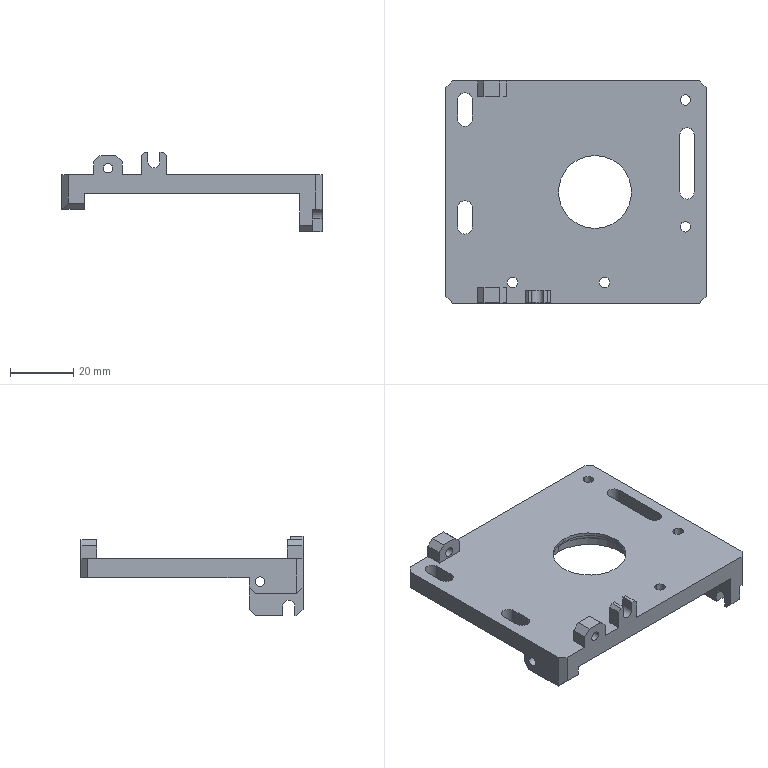NC program | NX | posted with a generic post | part box 82 x 70 x 25 mm
Lines 4706 to 5778 of 8354:
(FIXED_CONTOUR_COPY , TOOL : R1)
N9368 T02 M6
N9370 G54
N9372 G17 G0 G90 X-30.6 Y34.099 S9500 M3
N9374 G43 Z30. H2
N9376 Z2.8
N9378 G94 G1 Z0. F2800.
N9380 X-30.341 Z-0.034
N9382 X-30.1 Z-0.134
N9384 X-29.893 Z-0.293
N9386 X-29.734 Z-0.5
N9388 X-29.634 Z-0.741
N9390 X-29.6 Z-1.
N9392 Z-3.975
N9394 X-29.607 Z-4.096
N9396 X-29.613 Z-4.141
N9398 X-29.653 Z-4.278
N9400 X-29.706 Z-4.405
N9402 X-29.76 Z-4.502
N9404 X-29.813 Z-4.567
N9406 X-29.883 Z-4.646
N9408 X-29.953 Z-4.704
N9410 X-30.095 Z-4.794
N9412 X-30.233 Z-4.85
N9414 X-30.373 Z-4.889
N9416 X-30.517 Z-4.898
N9418 X-30.653 Z-4.885
N9420 X-30.793 Z-4.842
N9422 X-30.933 Z-4.779
N9424 X-31.003 Z-4.74
N9426 X-31.073 Z-4.682
N9428 X-31.143 Z-4.621
N9430 X-31.213 Z-4.536
N9432 X-31.306 Z-4.381
N9434 X-31.353 Z-4.256
N9436 X-31.377 Z-4.179
N9438 X-31.388 Z-4.13
N9440 X-31.394 Z-4.09
N9442 X-31.4 Z-3.975
N9444 Z-1.61
N9446 Y34.123 Z-1.
N9448 Y34.199
N9450 Z-3.975
N9452 X-31.394 Z-4.09
N9454 X-31.388 Z-4.13
N9456 X-31.377 Z-4.179
N9458 X-31.353 Z-4.256
N9460 X-31.306 Z-4.381
N9462 X-31.213 Z-4.536
N9464 X-31.143 Z-4.621
N9466 X-31.073 Z-4.682
N9468 X-31.003 Z-4.74
N9470 X-30.933 Z-4.779
N9472 X-30.793 Z-4.842
N9474 X-30.653 Z-4.885
N9476 X-30.513 Z-4.898
N9478 X-30.373 Z-4.889
N9480 X-30.233 Z-4.85
N9482 X-30.094 Z-4.793
N9484 X-29.953 Z-4.704
N9486 X-29.883 Z-4.646
N9488 X-29.813 Z-4.567
N9490 X-29.76 Z-4.502
N9492 X-29.706 Z-4.405
N9494 X-29.653 Z-4.278
N9496 X-29.613 Z-4.141
N9498 X-29.607 Z-4.096
N9500 X-29.6 Z-3.975
N9502 Z-1.
N9504 Y34.299
N9506 Z-3.975
N9508 X-29.607 Z-4.096
N9510 X-29.613 Z-4.141
N9512 X-29.653 Z-4.278
N9514 X-29.706 Z-4.405
N9516 X-29.76 Z-4.502
N9518 X-29.813 Z-4.567
N9520 X-29.883 Z-4.646
N9522 X-29.953 Z-4.704
N9524 X-30.093 Z-4.793
N9526 X-30.233 Z-4.85
N9528 X-30.373 Z-4.889
N9530 X-30.513 Z-4.898
N9532 X-30.653 Z-4.885
N9534 X-30.793 Z-4.842
N9536 X-30.933 Z-4.779
N9538 X-31.003 Z-4.74
N9540 X-31.073 Z-4.682
N9542 X-31.143 Z-4.621
N9544 X-31.213 Z-4.536
N9546 X-31.306 Z-4.381
N9548 X-31.353 Z-4.256
N9550 X-31.377 Z-4.179
N9552 X-31.388 Z-4.13
N9554 X-31.394 Z-4.09
N9556 X-31.4 Z-3.975
N9558 Z-1.
N9560 Y34.399
N9562 Z-3.975
N9564 X-31.394 Z-4.09
N9566 X-31.388 Z-4.13
N9568 X-31.377 Z-4.179
N9570 X-31.353 Z-4.256
N9572 X-31.306 Z-4.381
N9574 X-31.213 Z-4.536
N9576 X-31.143 Z-4.621
N9578 X-31.073 Z-4.682
N9580 X-31.003 Z-4.74
N9582 X-30.933 Z-4.779
N9584 X-30.793 Z-4.842
N9586 X-30.653 Z-4.885
N9588 X-30.513 Z-4.898
N9590 X-30.373 Z-4.889
N9592 X-30.233 Z-4.85
N9594 X-30.093 Z-4.793
N9596 X-29.953 Z-4.704
N9598 X-29.883 Z-4.646
N9600 X-29.813 Z-4.567
N9602 X-29.76 Z-4.502
N9604 X-29.706 Z-4.405
N9606 X-29.653 Z-4.278
N9608 X-29.613 Z-4.141
N9610 X-29.607 Z-4.096
N9612 X-29.6 Z-3.975
N9614 Z-1.
N9616 Y34.499
N9618 Z-3.975
N9620 X-29.607 Z-4.096
N9622 X-29.613 Z-4.141
N9624 X-29.653 Z-4.278
N9626 X-29.706 Z-4.405
N9628 X-29.76 Z-4.502
N9630 X-29.813 Z-4.567
N9632 X-29.883 Z-4.646
N9634 X-29.953 Z-4.704
N9636 X-30.093 Z-4.793
N9638 X-30.233 Z-4.85
N9640 X-30.373 Z-4.889
N9642 X-30.513 Z-4.898
N9644 X-30.653 Z-4.885
N9646 X-30.793 Z-4.842
N9648 X-30.933 Z-4.779
N9650 X-31.003 Z-4.74
N9652 X-31.073 Z-4.682
N9654 X-31.143 Z-4.621
N9656 X-31.213 Z-4.536
N9658 X-31.306 Z-4.381
N9660 X-31.353 Z-4.256
N9662 X-31.377 Z-4.179
N9664 X-31.388 Z-4.13
N9666 X-31.394 Z-4.09
N9668 X-31.4 Z-3.975
N9670 Z-1.
N9672 Y34.599
N9674 Z-3.975
N9676 X-31.394 Z-4.09
N9678 X-31.388 Z-4.13
N9680 X-31.377 Z-4.179
N9682 X-31.353 Z-4.256
N9684 X-31.306 Z-4.381
N9686 X-31.213 Z-4.536
N9688 X-31.143 Z-4.621
N9690 X-31.073 Z-4.682
N9692 X-31.003 Z-4.74
N9694 X-30.933 Z-4.779
N9696 X-30.793 Z-4.842
N9698 X-30.653 Z-4.885
N9700 X-30.513 Z-4.898
N9702 X-30.373 Z-4.889
N9704 X-30.233 Z-4.85
N9706 X-30.093 Z-4.793
N9708 X-29.953 Z-4.704
N9710 X-29.883 Z-4.646
N9712 X-29.813 Z-4.567
N9714 X-29.76 Z-4.502
N9716 X-29.706 Z-4.405
N9718 X-29.653 Z-4.278
N9720 X-29.613 Z-4.141
N9722 X-29.607 Z-4.096
N9724 X-29.6 Z-3.975
N9726 Z-1.
N9728 Y34.699
N9730 Z-3.975
N9732 X-29.607 Z-4.096
N9734 X-29.613 Z-4.141
N9736 X-29.653 Z-4.278
N9738 X-29.706 Z-4.405
N9740 X-29.76 Z-4.502
N9742 X-29.813 Z-4.567
N9744 X-29.883 Z-4.646
N9746 X-29.953 Z-4.704
N9748 X-30.093 Z-4.793
N9750 X-30.233 Z-4.85
N9752 X-30.373 Z-4.889
N9754 X-30.513 Z-4.898
N9756 X-30.653 Z-4.885
N9758 X-30.793 Z-4.842
N9760 X-30.933 Z-4.779
N9762 X-31.003 Z-4.74
N9764 X-31.073 Z-4.682
N9766 X-31.143 Z-4.621
N9768 X-31.213 Z-4.536
N9770 X-31.306 Z-4.381
N9772 X-31.353 Z-4.256
N9774 X-31.377 Z-4.179
N9776 X-31.388 Z-4.13
N9778 X-31.394 Z-4.09
N9780 X-31.4 Z-3.975
N9782 Z-1.
N9784 Y34.799
N9786 Z-3.975
N9788 X-31.394 Z-4.09
N9790 X-31.388 Z-4.13
N9792 X-31.377 Z-4.179
N9794 X-31.353 Z-4.256
N9796 X-31.306 Z-4.381
N9798 X-31.213 Z-4.536
N9800 X-31.143 Z-4.621
N9802 X-31.073 Z-4.682
N9804 X-31.003 Z-4.74
N9806 X-30.933 Z-4.779
N9808 X-30.793 Z-4.842
N9810 X-30.653 Z-4.885
N9812 X-30.513 Z-4.898
N9814 X-30.373 Z-4.889
N9816 X-30.233 Z-4.85
N9818 X-30.093 Z-4.793
N9820 X-29.953 Z-4.704
N9822 X-29.883 Z-4.646
N9824 X-29.813 Z-4.567
N9826 X-29.76 Z-4.502
N9828 X-29.706 Z-4.405
N9830 X-29.653 Z-4.278
N9832 X-29.613 Z-4.141
N9834 X-29.607 Z-4.096
N9836 X-29.6 Z-3.975
N9838 Z-1.
N9840 Y34.899
N9842 Z-3.975
N9844 X-29.607 Z-4.096
N9846 X-29.613 Z-4.141
N9848 X-29.653 Z-4.278
N9850 X-29.706 Z-4.405
N9852 X-29.76 Z-4.502
N9854 X-29.813 Z-4.567
N9856 X-29.883 Z-4.646
N9858 X-29.953 Z-4.704
N9860 X-30.093 Z-4.793
N9862 X-30.233 Z-4.85
N9864 X-30.373 Z-4.889
N9866 X-30.513 Z-4.898
N9868 X-30.653 Z-4.885
N9870 X-30.793 Z-4.842
N9872 X-30.933 Z-4.779
N9874 X-31.003 Z-4.74
N9876 X-31.073 Z-4.682
N9878 X-31.143 Z-4.621
N9880 X-31.213 Z-4.536
N9882 X-31.306 Z-4.381
N9884 X-31.353 Z-4.256
N9886 X-31.377 Z-4.179
N9888 X-31.388 Z-4.13
N9890 X-31.394 Z-4.09
N9892 X-31.4 Z-3.975
N9894 Z-1.
N9896 Y34.999
N9898 Z-3.975
N9900 X-31.394 Z-4.09
N9902 X-31.388 Z-4.13
N9904 X-31.377 Z-4.179
N9906 X-31.353 Z-4.256
N9908 X-31.306 Z-4.381
N9910 X-31.213 Z-4.536
N9912 X-31.143 Z-4.621
N9914 X-31.073 Z-4.682
N9916 X-31.003 Z-4.74
N9918 X-30.933 Z-4.779
N9920 X-30.793 Z-4.842
N9922 X-30.653 Z-4.885
N9924 X-30.513 Z-4.898
N9926 X-30.373 Z-4.889
N9928 X-30.233 Z-4.85
N9930 X-30.093 Z-4.793
N9932 X-29.953 Z-4.704
N9934 X-29.883 Z-4.646
N9936 X-29.813 Z-4.567
N9938 X-29.76 Z-4.502
N9940 X-29.706 Z-4.405
N9942 X-29.653 Z-4.278
N9944 X-29.613 Z-4.141
N9946 X-29.607 Z-4.096
N9948 X-29.6 Z-3.975
N9950 Z-1.
N9952 Y35.099
N9954 Z-3.975
N9956 X-29.607 Z-4.096
N9958 X-29.613 Z-4.141
N9960 X-29.653 Z-4.278
N9962 X-29.706 Z-4.405
N9964 X-29.76 Z-4.502
N9966 X-29.813 Z-4.567
N9968 X-29.883 Z-4.646
N9970 X-29.953 Z-4.704
N9972 X-30.093 Z-4.793
N9974 X-30.233 Z-4.85
N9976 X-30.373 Z-4.889
N9978 X-30.513 Z-4.898
N9980 X-30.653 Z-4.885
N9982 X-30.793 Z-4.842
N9984 X-30.933 Z-4.779
N9986 X-31.003 Z-4.74
N9988 X-31.073 Z-4.682
N9990 X-31.143 Z-4.621
N9992 X-31.213 Z-4.536
N9994 X-31.306 Z-4.381
N9996 X-31.353 Z-4.256
N9998 X-31.377 Z-4.179
N10000 X-31.388 Z-4.13
N10002 X-31.394 Z-4.09
N10004 X-31.4 Z-3.975
N10006 Z-1.
N10008 Y35.199
N10010 Z-3.975
N10012 X-31.394 Z-4.09
N10014 X-31.388 Z-4.13
N10016 X-31.377 Z-4.179
N10018 X-31.353 Z-4.256
N10020 X-31.306 Z-4.381
N10022 X-31.213 Z-4.536
N10024 X-31.143 Z-4.621
N10026 X-31.073 Z-4.682
N10028 X-31.003 Z-4.74
N10030 X-30.933 Z-4.779
N10032 X-30.793 Z-4.842
N10034 X-30.653 Z-4.885
N10036 X-30.513 Z-4.898
N10038 X-30.373 Z-4.889
N10040 X-30.233 Z-4.85
N10042 X-30.093 Z-4.793
N10044 X-29.953 Z-4.704
N10046 X-29.883 Z-4.646
N10048 X-29.813 Z-4.567
N10050 X-29.76 Z-4.502
N10052 X-29.706 Z-4.405
N10054 X-29.653 Z-4.278
N10056 X-29.613 Z-4.141
N10058 X-29.607 Z-4.096
N10060 X-29.6 Z-3.975
N10062 Z-1.
N10064 Y35.299
N10066 Z-3.975
N10068 X-29.607 Z-4.096
N10070 X-29.613 Z-4.141
N10072 X-29.653 Z-4.278
N10074 X-29.706 Z-4.405
N10076 X-29.76 Z-4.502
N10078 X-29.813 Z-4.567
N10080 X-29.883 Z-4.646
N10082 X-29.953 Z-4.704
N10084 X-30.093 Z-4.793
N10086 X-30.233 Z-4.85
N10088 X-30.373 Z-4.889
N10090 X-30.513 Z-4.898
N10092 X-30.653 Z-4.885
N10094 X-30.793 Z-4.842
N10096 X-30.933 Z-4.779
N10098 X-31.003 Z-4.74
N10100 X-31.073 Z-4.682
N10102 X-31.143 Z-4.621
N10104 X-31.213 Z-4.536
N10106 X-31.306 Z-4.381
N10108 X-31.353 Z-4.256
N10110 X-31.377 Z-4.179
N10112 X-31.388 Z-4.13
N10114 X-31.394 Z-4.09
N10116 X-31.4 Z-3.975
N10118 Z-1.
N10120 Y35.399
N10122 Z-3.975
N10124 X-31.394 Z-4.09
N10126 X-31.388 Z-4.129
N10128 X-31.377 Z-4.178
N10130 X-31.353 Z-4.256
N10132 X-31.306 Z-4.381
N10134 X-31.213 Z-4.536
N10136 X-31.143 Z-4.621
N10138 X-31.075 Z-4.681
N10140 X-31.003 Z-4.74
N10142 X-30.933 Z-4.779
N10144 X-30.793 Z-4.842
N10146 X-30.653 Z-4.885
N10148 X-30.513 Z-4.898
N10150 X-30.373 Z-4.889
N10152 X-30.233 Z-4.85
N10154 X-30.093 Z-4.793
N10156 X-29.953 Z-4.704
N10158 X-29.883 Z-4.646
N10160 X-29.815 Z-4.569
N10162 X-29.76 Z-4.502
N10164 X-29.706 Z-4.405
N10166 X-29.653 Z-4.278
N10168 X-29.613 Z-4.141
N10170 X-29.607 Z-4.097
N10172 X-29.6 Z-3.976
N10174 Z-1.
N10176 Y35.499
N10178 Z-3.975
N10180 X-29.607 Z-4.096
N10182 X-29.613 Z-4.141
N10184 X-29.653 Z-4.278
N10186 X-29.706 Z-4.405
N10188 X-29.76 Z-4.502
N10190 X-29.813 Z-4.567
N10192 X-29.883 Z-4.646
N10194 X-29.953 Z-4.704
N10196 X-30.093 Z-4.793
N10198 X-30.233 Z-4.85
N10200 X-30.373 Z-4.889
N10202 X-30.513 Z-4.898
N10204 X-30.653 Z-4.885
N10206 X-30.793 Z-4.842
N10208 X-30.933 Z-4.779
N10210 X-31.003 Z-4.74
N10212 X-31.073 Z-4.682
N10214 X-31.143 Z-4.621
N10216 X-31.213 Z-4.536
N10218 X-31.306 Z-4.381
N10220 X-31.353 Z-4.256
N10222 X-31.377 Z-4.179
N10224 X-31.388 Z-4.13
N10226 X-31.394 Z-4.09
N10228 X-31.4 Z-3.975
N10230 Z-1.
N10232 Y35.599
N10234 Z-3.975
N10236 X-31.394 Z-4.09
N10238 X-31.388 Z-4.13
N10240 X-31.377 Z-4.179
N10242 X-31.353 Z-4.256
N10244 X-31.306 Z-4.381
N10246 X-31.213 Z-4.536
N10248 X-31.143 Z-4.621
N10250 X-31.073 Z-4.682
N10252 X-31.003 Z-4.74
N10254 X-30.933 Z-4.779
N10256 X-30.793 Z-4.842
N10258 X-30.653 Z-4.885
N10260 X-30.513 Z-4.898
N10262 X-30.373 Z-4.889
N10264 X-30.233 Z-4.85
N10266 X-30.093 Z-4.793
N10268 X-29.953 Z-4.704
N10270 X-29.883 Z-4.646
N10272 X-29.813 Z-4.567
N10274 X-29.76 Z-4.502
N10276 X-29.706 Z-4.405
N10278 X-29.653 Z-4.278
N10280 X-29.613 Z-4.141
N10282 X-29.607 Z-4.096
N10284 X-29.6 Z-3.975
N10286 Z-1.
N10288 Y35.699
N10290 Z-3.975
N10292 X-29.607 Z-4.096
N10294 X-29.613 Z-4.141
N10296 X-29.653 Z-4.278
N10298 X-29.706 Z-4.405
N10300 X-29.76 Z-4.502
N10302 X-29.813 Z-4.567
N10304 X-29.883 Z-4.646
N10306 X-29.953 Z-4.704
N10308 X-30.093 Z-4.793
N10310 X-30.233 Z-4.85
N10312 X-30.373 Z-4.889
N10314 X-30.513 Z-4.898
N10316 X-30.653 Z-4.885
N10318 X-30.793 Z-4.842
N10320 X-30.933 Z-4.779
N10322 X-31.003 Z-4.74
N10324 X-31.073 Z-4.682
N10326 X-31.143 Z-4.621
N10328 X-31.213 Z-4.536
N10330 X-31.306 Z-4.381
N10332 X-31.353 Z-4.256
N10334 X-31.377 Z-4.179
N10336 X-31.388 Z-4.13
N10338 X-31.394 Z-4.09
N10340 X-31.4 Z-3.975
N10342 Z-1.
N10344 Y35.799
N10346 Z-3.975
N10348 X-31.394 Z-4.09
N10350 X-31.388 Z-4.13
N10352 X-31.377 Z-4.179
N10354 X-31.353 Z-4.256
N10356 X-31.306 Z-4.381
N10358 X-31.213 Z-4.536
N10360 X-31.143 Z-4.621
N10362 X-31.073 Z-4.682
N10364 X-31.003 Z-4.74
N10366 X-30.933 Z-4.779
N10368 X-30.793 Z-4.842
N10370 X-30.653 Z-4.885
N10372 X-30.513 Z-4.898
N10374 X-30.373 Z-4.889
N10376 X-30.233 Z-4.85
N10378 X-30.093 Z-4.793
N10380 X-29.953 Z-4.704
N10382 X-29.883 Z-4.646
N10384 X-29.813 Z-4.567
N10386 X-29.76 Z-4.502
N10388 X-29.706 Z-4.405
N10390 X-29.653 Z-4.278
N10392 X-29.613 Z-4.141
N10394 X-29.607 Z-4.096
N10396 X-29.6 Z-3.975
N10398 Z-1.
N10400 Y35.899
N10402 Z-3.975
N10404 X-29.607 Z-4.096
N10406 X-29.613 Z-4.141
N10408 X-29.653 Z-4.278
N10410 X-29.706 Z-4.405
N10412 X-29.76 Z-4.502
N10414 X-29.813 Z-4.567
N10416 X-29.883 Z-4.646
N10418 X-29.953 Z-4.704
N10420 X-30.093 Z-4.793
N10422 X-30.233 Z-4.85
N10424 X-30.373 Z-4.889
N10426 X-30.513 Z-4.898
N10428 X-30.653 Z-4.885
N10430 X-30.793 Z-4.842
N10432 X-30.933 Z-4.779
N10434 X-31.003 Z-4.74
N10436 X-31.073 Z-4.682
N10438 X-31.143 Z-4.621
N10440 X-31.213 Z-4.536
N10442 X-31.306 Z-4.381
N10444 X-31.353 Z-4.256
N10446 X-31.377 Z-4.179
N10448 X-31.388 Z-4.13
N10450 X-31.394 Z-4.09
N10452 X-31.4 Z-3.975
N10454 Z-1.
N10456 Y35.999
N10458 Z-3.975
N10460 X-31.394 Z-4.09
N10462 X-31.388 Z-4.13
N10464 X-31.377 Z-4.179
N10466 X-31.353 Z-4.256
N10468 X-31.306 Z-4.381
N10470 X-31.213 Z-4.536
N10472 X-31.143 Z-4.621
N10474 X-31.073 Z-4.682
N10476 X-31.003 Z-4.74
N10478 X-30.933 Z-4.779
N10480 X-30.793 Z-4.842
N10482 X-30.653 Z-4.885
N10484 X-30.513 Z-4.898
N10486 X-30.373 Z-4.889
N10488 X-30.233 Z-4.85
N10490 X-30.093 Z-4.793
N10492 X-29.953 Z-4.704
N10494 X-29.883 Z-4.646
N10496 X-29.813 Z-4.567
N10498 X-29.76 Z-4.502
N10500 X-29.706 Z-4.405
N10502 X-29.653 Z-4.278
N10504 X-29.613 Z-4.141
N10506 X-29.607 Z-4.096
N10508 X-29.6 Z-3.975
N10510 Z-1.
N10512 Y36.099
N10514 Z-3.975
N10516 X-29.607 Z-4.096
N10518 X-29.613 Z-4.141
N10520 X-29.653 Z-4.278
N10522 X-29.706 Z-4.405
N10524 X-29.76 Z-4.502
N10526 X-29.813 Z-4.567
N10528 X-29.883 Z-4.646
N10530 X-29.953 Z-4.704
N10532 X-30.093 Z-4.793
N10534 X-30.233 Z-4.85
N10536 X-30.373 Z-4.889
N10538 X-30.513 Z-4.898
N10540 X-30.653 Z-4.885
N10542 X-30.793 Z-4.842
N10544 X-30.933 Z-4.779
N10546 X-31.003 Z-4.74
N10548 X-31.073 Z-4.682
N10550 X-31.143 Z-4.621
N10552 X-31.213 Z-4.536
N10554 X-31.306 Z-4.381
N10556 X-31.353 Z-4.256
N10558 X-31.377 Z-4.179
N10560 X-31.388 Z-4.13
N10562 X-31.394 Z-4.09
N10564 X-31.4 Z-3.975
N10566 Z-1.
N10568 Y36.199
N10570 Z-3.975
N10572 X-31.394 Z-4.09
N10574 X-31.388 Z-4.13
N10576 X-31.377 Z-4.179
N10578 X-31.353 Z-4.256
N10580 X-31.306 Z-4.381
N10582 X-31.213 Z-4.536
N10584 X-31.143 Z-4.621
N10586 X-31.073 Z-4.682
N10588 X-31.003 Z-4.74
N10590 X-30.933 Z-4.779
N10592 X-30.793 Z-4.842
N10594 X-30.653 Z-4.885
N10596 X-30.513 Z-4.898
N10598 X-30.373 Z-4.889
N10600 X-30.233 Z-4.85
N10602 X-30.093 Z-4.793
N10604 X-29.953 Z-4.704
N10606 X-29.883 Z-4.646
N10608 X-29.813 Z-4.567
N10610 X-29.76 Z-4.502
N10612 X-29.706 Z-4.405
N10614 X-29.653 Z-4.278
N10616 X-29.613 Z-4.141
N10618 X-29.607 Z-4.096
N10620 X-29.6 Z-3.975
N10622 Z-1.
N10624 Y36.299
N10626 Z-3.975
N10628 X-29.607 Z-4.096
N10630 X-29.613 Z-4.141
N10632 X-29.653 Z-4.278
N10634 X-29.706 Z-4.405
N10636 X-29.76 Z-4.502
N10638 X-29.813 Z-4.567
N10640 X-29.883 Z-4.646
N10642 X-29.953 Z-4.704
N10644 X-30.093 Z-4.793
N10646 X-30.233 Z-4.85
N10648 X-30.373 Z-4.889
N10650 X-30.513 Z-4.898
N10652 X-30.653 Z-4.885
N10654 X-30.793 Z-4.842
N10656 X-30.933 Z-4.779
N10658 X-31.003 Z-4.74
N10660 X-31.073 Z-4.682
N10662 X-31.143 Z-4.621
N10664 X-31.213 Z-4.536
N10666 X-31.306 Z-4.381
N10668 X-31.353 Z-4.256
N10670 X-31.377 Z-4.179
N10672 X-31.388 Z-4.13
N10674 X-31.394 Z-4.09
N10676 X-31.4 Z-3.975
N10678 Z-1.
N10680 Y36.399
N10682 Z-3.975
N10684 X-31.394 Z-4.09
N10686 X-31.388 Z-4.13
N10688 X-31.377 Z-4.179
N10690 X-31.353 Z-4.256
N10692 X-31.306 Z-4.381
N10694 X-31.213 Z-4.536
N10696 X-31.143 Z-4.621
N10698 X-31.073 Z-4.682
N10700 X-31.003 Z-4.74
N10702 X-30.933 Z-4.779
N10704 X-30.793 Z-4.842
N10706 X-30.653 Z-4.885
N10708 X-30.513 Z-4.898
N10710 X-30.373 Z-4.889
N10712 X-30.233 Z-4.85
N10714 X-30.093 Z-4.793
N10716 X-29.953 Z-4.704
N10718 X-29.883 Z-4.646
N10720 X-29.813 Z-4.567
N10722 X-29.76 Z-4.502
N10724 X-29.706 Z-4.405
N10726 X-29.653 Z-4.278
N10728 X-29.613 Z-4.141
N10730 X-29.607 Z-4.096
N10732 X-29.6 Z-3.975
N10734 Z-1.
N10736 Y36.499
N10738 Z-3.975
N10740 X-29.607 Z-4.096
N10742 X-29.613 Z-4.141
N10744 X-29.653 Z-4.278
N10746 X-29.706 Z-4.405
N10748 X-29.76 Z-4.502
N10750 X-29.813 Z-4.567
N10752 X-29.883 Z-4.646
N10754 X-29.953 Z-4.704
N10756 X-30.093 Z-4.793
N10758 X-30.233 Z-4.85
N10760 X-30.373 Z-4.889
N10762 X-30.513 Z-4.898
N10764 X-30.653 Z-4.885
N10766 X-30.793 Z-4.842
N10768 X-30.933 Z-4.779
N10770 X-31.003 Z-4.74
N10772 X-31.073 Z-4.682
N10774 X-31.143 Z-4.621
N10776 X-31.213 Z-4.536
N10778 X-31.306 Z-4.381
N10780 X-31.353 Z-4.256
N10782 X-31.377 Z-4.179
N10784 X-31.388 Z-4.13
N10786 X-31.394 Z-4.09
N10788 X-31.4 Z-3.975
N10790 Z-1.
N10792 Y36.599
N10794 Z-3.975
N10796 X-31.394 Z-4.09
N10798 X-31.388 Z-4.13
N10800 X-31.377 Z-4.179
N10802 X-31.353 Z-4.256
N10804 X-31.306 Z-4.381
N10806 X-31.213 Z-4.536
N10808 X-31.143 Z-4.621
N10810 X-31.073 Z-4.682
N10812 X-31.003 Z-4.74
N10814 X-30.933 Z-4.779
N10816 X-30.793 Z-4.842
N10818 X-30.653 Z-4.885
N10820 X-30.513 Z-4.898
N10822 X-30.373 Z-4.889
N10824 X-30.233 Z-4.85
N10826 X-30.093 Z-4.793
N10828 X-29.953 Z-4.704
N10830 X-29.883 Z-4.646
N10832 X-29.813 Z-4.567
N10834 X-29.76 Z-4.502
N10836 X-29.706 Z-4.405
N10838 X-29.653 Z-4.278
N10840 X-29.613 Z-4.141
N10842 X-29.607 Z-4.096
N10844 X-29.6 Z-3.975
N10846 Z-1.
N10848 Y36.699
N10850 Z-3.975
N10852 X-29.607 Z-4.096
N10854 X-29.613 Z-4.141
N10856 X-29.653 Z-4.278
N10858 X-29.706 Z-4.405
N10860 X-29.76 Z-4.502
N10862 X-29.813 Z-4.567
N10864 X-29.883 Z-4.646
N10866 X-29.953 Z-4.704
N10868 X-30.093 Z-4.793
N10870 X-30.233 Z-4.85
N10872 X-30.373 Z-4.889
N10874 X-30.513 Z-4.898
N10876 X-30.653 Z-4.885
N10878 X-30.793 Z-4.842
N10880 X-30.933 Z-4.779
N10882 X-31.003 Z-4.74
N10884 X-31.073 Z-4.682
N10886 X-31.143 Z-4.621
N10888 X-31.213 Z-4.536
N10890 X-31.306 Z-4.381
N10892 X-31.353 Z-4.256
N10894 X-31.377 Z-4.179
N10896 X-31.388 Z-4.13
N10898 X-31.394 Z-4.09
N10900 X-31.4 Z-3.975
N10902 Z-1.
N10904 Y36.799
N10906 Z-3.975
N10908 X-31.394 Z-4.089
N10910 X-31.388 Z-4.129
N10912 X-31.377 Z-4.179
N10914 X-31.353 Z-4.255
N10916 X-31.306 Z-4.381
N10918 X-31.213 Z-4.536
N10920 X-31.143 Z-4.621
N10922 X-31.074 Z-4.682
N10924 X-31.003 Z-4.74
N10926 X-30.934 Z-4.778
N10928 X-30.793 Z-4.842
N10930 X-30.653 Z-4.885
N10932 X-30.513 Z-4.898
N10934 X-30.373 Z-4.889
N10936 X-30.233 Z-4.85
N10938 X-30.093 Z-4.793
N10940 X-29.953 Z-4.704
N10942 X-29.883 Z-4.646
N10944 X-29.814 Z-4.568
N10946 X-29.76 Z-4.502
N10948 X-29.706 Z-4.405
N10950 X-29.653 Z-4.278
N10952 X-29.613 Z-4.141
N10954 X-29.607 Z-4.096
N10956 X-29.6 Z-3.976
N10958 Z-1.
N10960 Y36.899
N10962 Z-3.975
N10964 X-29.607 Z-4.096
N10966 X-29.613 Z-4.141
N10968 X-29.653 Z-4.278
N10970 X-29.706 Z-4.405
N10972 X-29.76 Z-4.502
N10974 X-29.813 Z-4.567
N10976 X-29.883 Z-4.646
N10978 X-29.953 Z-4.704
N10980 X-30.093 Z-4.793
N10982 X-30.233 Z-4.85
N10984 X-30.373 Z-4.889
N10986 X-30.513 Z-4.898
N10988 X-30.653 Z-4.885
N10990 X-30.793 Z-4.842
N10992 X-30.933 Z-4.779
N10994 X-31.003 Z-4.74
N10996 X-31.073 Z-4.682
N10998 X-31.143 Z-4.621
N11000 X-31.213 Z-4.536
N11002 X-31.306 Z-4.381
N11004 X-31.353 Z-4.256
N11006 X-31.377 Z-4.179
N11008 X-31.388 Z-4.13
N11010 X-31.394 Z-4.09
N11012 X-31.4 Z-3.975
N11014 Z-1.
N11016 Y36.999
N11018 Z-3.975
N11020 X-31.394 Z-4.09
N11022 X-31.388 Z-4.13
N11024 X-31.377 Z-4.179
N11026 X-31.353 Z-4.256
N11028 X-31.306 Z-4.381
N11030 X-31.213 Z-4.536
N11032 X-31.143 Z-4.621
N11034 X-31.073 Z-4.682
N11036 X-31.003 Z-4.74
N11038 X-30.933 Z-4.779
N11040 X-30.793 Z-4.842
N11042 X-30.653 Z-4.885
N11044 X-30.513 Z-4.898
N11046 X-30.373 Z-4.889
N11048 X-30.233 Z-4.85
N11050 X-30.093 Z-4.793
N11052 X-29.953 Z-4.704
N11054 X-29.883 Z-4.646
N11056 X-29.813 Z-4.567
N11058 X-29.76 Z-4.502
N11060 X-29.706 Z-4.405
N11062 X-29.653 Z-4.278
N11064 X-29.613 Z-4.141
N11066 X-29.607 Z-4.096
N11068 X-29.6 Z-3.975
N11070 Z-1.
N11072 Y37.099
N11074 Z-3.975
N11076 X-29.607 Z-4.096
N11078 X-29.613 Z-4.141
N11080 X-29.653 Z-4.278
N11082 X-29.706 Z-4.405
N11084 X-29.76 Z-4.502
N11086 X-29.813 Z-4.567
N11088 X-29.883 Z-4.646
N11090 X-29.953 Z-4.704
N11092 X-30.093 Z-4.793
N11094 X-30.233 Z-4.85
N11096 X-30.373 Z-4.889
N11098 X-30.513 Z-4.898
N11100 X-30.653 Z-4.885
N11102 X-30.793 Z-4.842
N11104 X-30.933 Z-4.779
N11106 X-31.003 Z-4.74
N11108 X-31.073 Z-4.682
N11110 X-31.143 Z-4.621
N11112 X-31.213 Z-4.536
N11114 X-31.306 Z-4.381
N11116 X-31.353 Z-4.256
N11118 X-31.377 Z-4.179
N11120 X-31.388 Z-4.13
N11122 X-31.394 Z-4.09
N11124 X-31.4 Z-3.975
N11126 Z-1.
N11128 Y37.199
N11130 Z-3.975
N11132 X-31.394 Z-4.09
N11134 X-31.388 Z-4.13
N11136 X-31.377 Z-4.179
N11138 X-31.353 Z-4.256
N11140 X-31.306 Z-4.381
N11142 X-31.213 Z-4.536
N11144 X-31.143 Z-4.621
N11146 X-31.073 Z-4.682
N11148 X-31.003 Z-4.74
N11150 X-30.933 Z-4.779
N11152 X-30.793 Z-4.842
N11154 X-30.653 Z-4.885
N11156 X-30.513 Z-4.898
N11158 X-30.373 Z-4.889
N11160 X-30.233 Z-4.85
N11162 X-30.093 Z-4.793
N11164 X-29.953 Z-4.704
N11166 X-29.883 Z-4.646
N11168 X-29.813 Z-4.567
N11170 X-29.76 Z-4.502
N11172 X-29.706 Z-4.405
N11174 X-29.653 Z-4.278
N11176 X-29.613 Z-4.141
N11178 X-29.607 Z-4.096
N11180 X-29.6 Z-3.975
N11182 Z-1.
N11184 Y37.299
N11186 Z-3.975
N11188 X-29.607 Z-4.096
N11190 X-29.613 Z-4.141
N11192 X-29.653 Z-4.278
N11194 X-29.706 Z-4.405
N11196 X-29.76 Z-4.502
N11198 X-29.813 Z-4.567
N11200 X-29.883 Z-4.646
N11202 X-29.953 Z-4.704
N11204 X-30.093 Z-4.793
N11206 X-30.233 Z-4.85
N11208 X-30.373 Z-4.889
N11210 X-30.513 Z-4.898
N11212 X-30.653 Z-4.885
N11214 X-30.793 Z-4.842
N11216 X-30.933 Z-4.779
N11218 X-31.003 Z-4.74
N11220 X-31.073 Z-4.682
N11222 X-31.143 Z-4.621
N11224 X-31.213 Z-4.536
N11226 X-31.306 Z-4.381
N11228 X-31.353 Z-4.256
N11230 X-31.377 Z-4.179
N11232 X-31.388 Z-4.13
N11234 X-31.394 Z-4.09
N11236 X-31.4 Z-3.975
N11238 Z-1.
N11240 Y37.399
N11242 Z-3.975
N11244 X-31.394 Z-4.09
N11246 X-31.388 Z-4.13
N11248 X-31.377 Z-4.179
N11250 X-31.353 Z-4.256
N11252 X-31.306 Z-4.381
N11254 X-31.213 Z-4.536
N11256 X-31.143 Z-4.621
N11258 X-31.073 Z-4.682
N11260 X-31.003 Z-4.74
N11262 X-30.933 Z-4.779
N11264 X-30.793 Z-4.842
N11266 X-30.653 Z-4.885
N11268 X-30.513 Z-4.898
N11270 X-30.373 Z-4.889
N11272 X-30.233 Z-4.85
N11274 X-30.093 Z-4.793
N11276 X-29.953 Z-4.704
N11278 X-29.883 Z-4.646
N11280 X-29.813 Z-4.567
N11282 X-29.76 Z-4.502
N11284 X-29.706 Z-4.405
N11286 X-29.653 Z-4.278
N11288 X-29.613 Z-4.141
N11290 X-29.607 Z-4.096
N11292 X-29.6 Z-3.975
N11294 Z-1.
N11296 Y37.499
N11298 Z-3.975
N11300 X-29.607 Z-4.096
N11302 X-29.613 Z-4.141
N11304 X-29.653 Z-4.278
N11306 X-29.706 Z-4.405
N11308 X-29.76 Z-4.502
N11310 X-29.813 Z-4.567
N11312 X-29.883 Z-4.646
N11314 X-29.953 Z-4.704
N11316 X-30.093 Z-4.793
N11318 X-30.233 Z-4.85
N11320 X-30.373 Z-4.889
N11322 X-30.513 Z-4.898
N11324 X-30.653 Z-4.885
N11326 X-30.793 Z-4.842
N11328 X-30.933 Z-4.779
N11330 X-31.003 Z-4.74
N11332 X-31.073 Z-4.682
N11334 X-31.143 Z-4.621
N11336 X-31.213 Z-4.536
N11338 X-31.306 Z-4.381
N11340 X-31.353 Z-4.256
N11342 X-31.377 Z-4.179
N11344 X-31.388 Z-4.13
N11346 X-31.394 Z-4.09
N11348 X-31.4 Z-3.975
N11350 Z-1.
N11352 Y37.599
N11354 Z-3.975
N11356 X-31.394 Z-4.09
N11358 X-31.388 Z-4.13
N11360 X-31.377 Z-4.179
N11362 X-31.353 Z-4.256
N11364 X-31.306 Z-4.381
N11366 X-31.213 Z-4.536
N11368 X-31.143 Z-4.621
N11370 X-31.073 Z-4.682
N11372 X-31.003 Z-4.74
N11374 X-30.933 Z-4.779
N11376 X-30.793 Z-4.842
N11378 X-30.653 Z-4.885
N11380 X-30.513 Z-4.898
N11382 X-30.373 Z-4.889
N11384 X-30.233 Z-4.85
N11386 X-30.093 Z-4.793
N11388 X-29.953 Z-4.704
N11390 X-29.883 Z-4.646
N11392 X-29.813 Z-4.567
N11394 X-29.76 Z-4.502
N11396 X-29.706 Z-4.405
N11398 X-29.653 Z-4.278
N11400 X-29.613 Z-4.141
N11402 X-29.607 Z-4.096
N11404 X-29.6 Z-3.975
N11406 Z-1.
N11408 Y37.699
N11410 Z-3.975
N11412 X-29.607 Z-4.096
N11414 X-29.613 Z-4.141
N11416 X-29.653 Z-4.278
N11418 X-29.706 Z-4.405
N11420 X-29.76 Z-4.502
N11422 X-29.813 Z-4.567
N11424 X-29.883 Z-4.646
N11426 X-29.953 Z-4.704
N11428 X-30.093 Z-4.793
N11430 X-30.233 Z-4.85
N11432 X-30.373 Z-4.889
N11434 X-30.513 Z-4.898
N11436 X-30.653 Z-4.885
N11438 X-30.793 Z-4.842
N11440 X-30.933 Z-4.779
N11442 X-31.003 Z-4.74
N11444 X-31.073 Z-4.682
N11446 X-31.143 Z-4.621
N11448 X-31.213 Z-4.536
N11450 X-31.306 Z-4.381
N11452 X-31.353 Z-4.256
N11454 X-31.377 Z-4.179
N11456 X-31.388 Z-4.13
N11458 X-31.394 Z-4.09
N11460 X-31.4 Z-3.975
N11462 Z-1.
N11464 Y37.799
N11466 Z-3.975
N11468 X-31.394 Z-4.09
N11470 X-31.388 Z-4.13
N11472 X-31.377 Z-4.179
N11474 X-31.353 Z-4.256
N11476 X-31.306 Z-4.381
N11478 X-31.213 Z-4.536
N11480 X-31.143 Z-4.621
N11482 X-31.073 Z-4.682
N11484 X-31.003 Z-4.74
N11486 X-30.933 Z-4.779
N11488 X-30.793 Z-4.842
N11490 X-30.653 Z-4.885
N11492 X-30.513 Z-4.898
N11494 X-30.373 Z-4.889
N11496 X-30.233 Z-4.85
N11498 X-30.093 Z-4.793
N11500 X-29.953 Z-4.704
N11502 X-29.883 Z-4.646
N11504 X-29.813 Z-4.567
N11506 X-29.76 Z-4.502